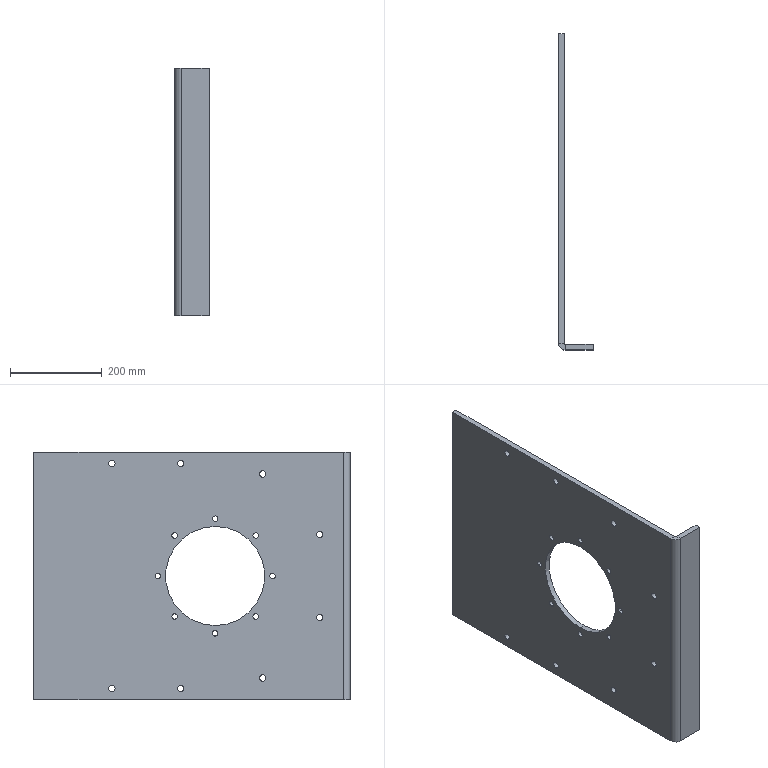Part | STEP file | Input 54 | 1 solid | 48 faces | box 75 x 689 x 540 mm | volume 4383962 mm3 | cylinder 36 | plane 12 | commonest cylinder face diameters 12 x16 14 x16 216 x2 5 x1 29 x1